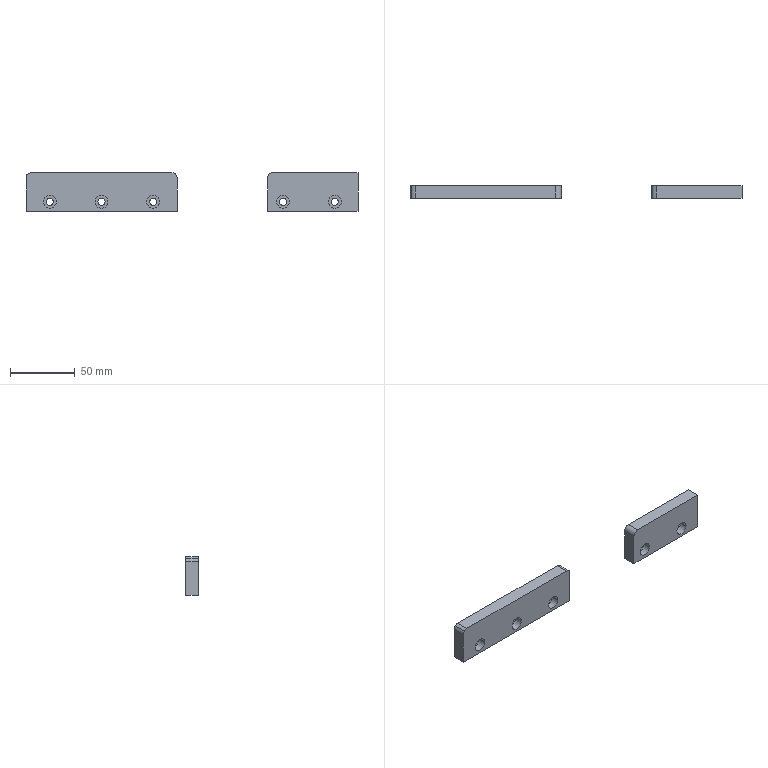Part | STEP file | ASND-0110-TCTF01-58 | 2 solids | 41 faces | box 256.83 x 10 x 30 mm | volume 53115 mm3 | cylinder 24 | plane 17 | commonest cylinder face diameters 5.5 x10 10 x10 8 x4